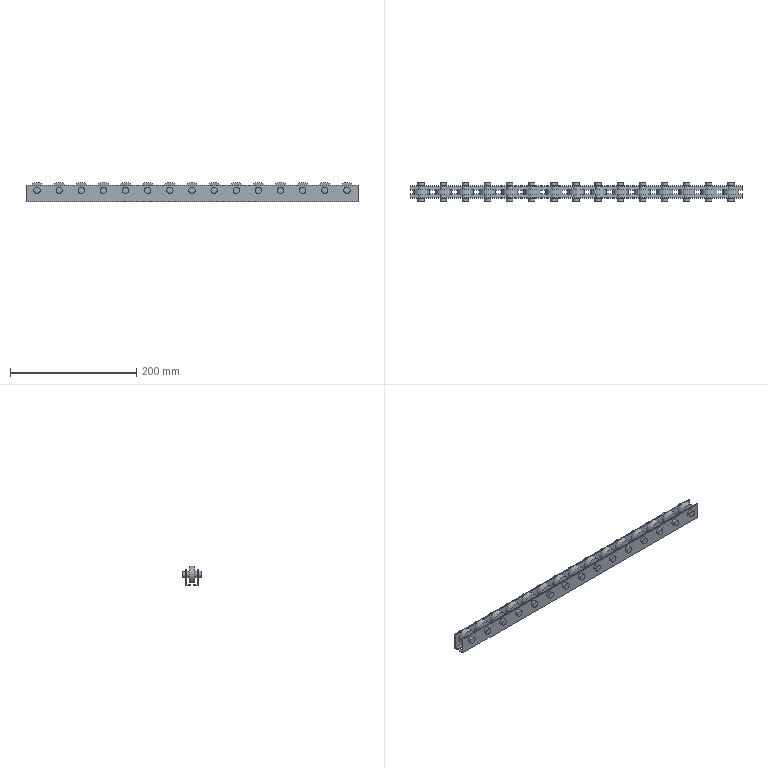Part | NX | features solid 2 | 1 solid | 151 faces | box 525 x 29 x 30.5 mm | volume 140950 mm3 | plane 76 | cylinder 75 | commonest cylinder face diameters 10 x60 25.4 x15